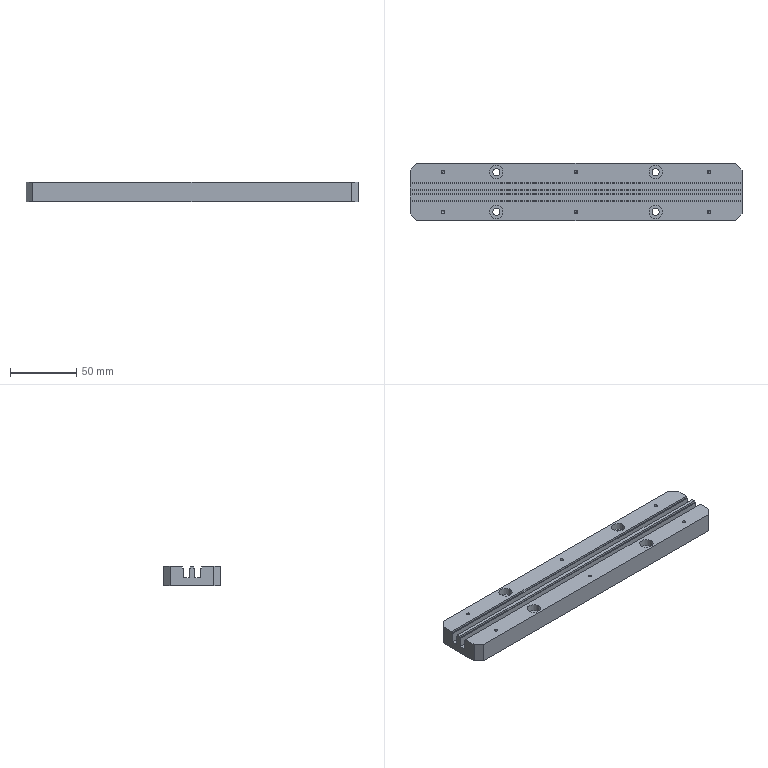Part | STEP file | B01 | 1 solid | 70 faces | box 250 x 43 x 15 mm | volume 136288 mm3 | plane 30 | cylinder 28 | cone 12 | commonest cylinder face diameters 2.5 x12 5.5 x8 10 x8